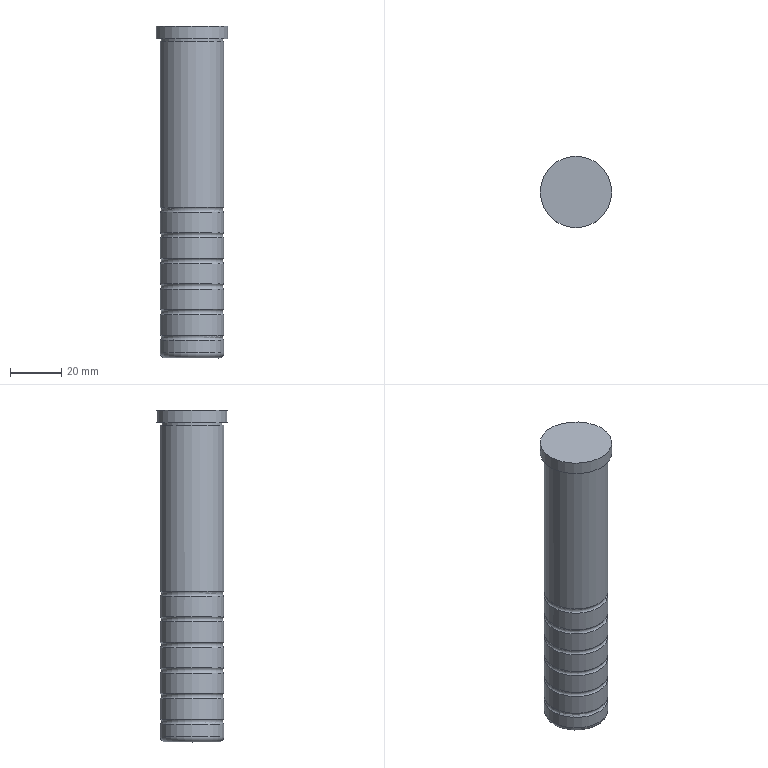Part | NX | features SGOH25-130 2 | 1 solid | 20 faces | box 28 x 28 x 130 mm | volume 64011 mm3 | cylinder 9 | torus 7 | plane 4 | commonest cylinder face diameters 25 x7 24 x1 28 x1
STEP:
#1=CARTESIAN_POINT('',(3690.594,-749.195,874.716));
#2=VERTEX_POINT('',#1);
#3=CARTESIAN_POINT('',(3703.094,-749.122,874.716));
#4=DIRECTION('',(0.,0.,1.));
#5=DIRECTION('',(1.,0.,0.));
#6=AXIS2_PLACEMENT_3D('',#3,#4,#5);
#7=CIRCLE('',#6,12.5);
#8=EDGE_CURVE('',#2,#2,#7,.T.);
#9=ORIENTED_EDGE('',*,*,#8,.T.);
#10=EDGE_LOOP('',(#9));
#11=FACE_BOUND('',#10,.T.);
#12=CARTESIAN_POINT('',(3690.594,-749.122,939.716));
#13=VERTEX_POINT('',#12);
#14=CARTESIAN_POINT('',(3703.094,-749.122,939.716));
#15=DIRECTION('',(0.,0.,-1.));
#16=DIRECTION('',(-1.,0.,0.));
#17=AXIS2_PLACEMENT_3D('',#14,#15,#16);
#18=CIRCLE('',#17,12.5);
#19=EDGE_CURVE('',#13,#13,#18,.T.);
#20=ORIENTED_EDGE('',*,*,#19,.T.);
#21=EDGE_LOOP('',(#20));
#22=FACE_BOUND('',#21,.T.);
#23=CARTESIAN_POINT('',(3703.094,-749.122,880.716));
#24=DIRECTION('',(0.,0.,-1.));
#25=DIRECTION('',(0.008727,-1.,0.));
#26=AXIS2_PLACEMENT_3D('',#23,#24,#25);
#27=CYLINDRICAL_SURFACE('',#26,12.5);
#28=ADVANCED_FACE('',(#11,#22),#27,.T.);
#29=CARTESIAN_POINT('',(3691.094,-749.122,940.716));
#30=VERTEX_POINT('',#29);
#31=CARTESIAN_POINT('',(3703.094,-749.122,940.716));
#32=DIRECTION('',(0.,0.,-1.));
#33=DIRECTION('',(-1.,0.,0.));
#34=AXIS2_PLACEMENT_3D('',#31,#32,#33);
#35=CIRCLE('',#34,12.);
#36=EDGE_CURVE('',#30,#30,#35,.T.);
#37=ORIENTED_EDGE('',*,*,#36,.T.);
#38=CARTESIAN_POINT('',(3691.094,-749.122,939.716));
#39=VERTEX_POINT('',#38);
#40=CARTESIAN_POINT('',(3691.094,-749.122,940.216));
#41=DIRECTION('',(0.,0.,-1.));
#42=VECTOR('',#41,1000.);
#43=LINE('',#40,#42);
#44=EDGE_CURVE('',#30,#39,#43,.T.);
#45=ORIENTED_EDGE('',*,*,#44,.T.);
#46=CARTESIAN_POINT('',(3703.094,-749.122,939.716));
#47=DIRECTION('',(0.,0.,1.));
#48=DIRECTION('',(-1.,0.,0.));
#49=AXIS2_PLACEMENT_3D('',#46,#47,#48);
#50=CIRCLE('',#49,12.);
#51=EDGE_CURVE('',#39,#39,#50,.T.);
#52=ORIENTED_EDGE('',*,*,#51,.T.);
#53=ORIENTED_EDGE('',*,*,#44,.F.);
#54=EDGE_LOOP('',(#37,#45,#52,#53));
#55=FACE_BOUND('',#54,.T.);
#56=CARTESIAN_POINT('',(3703.094,-749.122,940.216));
#57=DIRECTION('',(0.,0.,-1.));
#58=DIRECTION('',(1.,0.,0.));
#59=AXIS2_PLACEMENT_3D('',#56,#57,#58);
#60=CYLINDRICAL_SURFACE('',#59,12.);
#61=ADVANCED_FACE('',(#55),#60,.T.);
#62=ORIENTED_EDGE('',*,*,#19,.F.);
#63=EDGE_LOOP('',(#62));
#64=FACE_BOUND('',#63,.T.);
#65=ORIENTED_EDGE('',*,*,#51,.F.);
#66=EDGE_LOOP('',(#65));
#67=FACE_BOUND('',#66,.T.);
#68=CARTESIAN_POINT('',(3731.844,-775.103,939.716));
#69=DIRECTION('',(0.,0.,-1.));
#70=DIRECTION('',(1.,0.,0.));
#71=AXIS2_PLACEMENT_3D('',#68,#69,#70);
#72=PLANE('',#71);
#73=ADVANCED_FACE('',(#64,#67),#72,.F.);
#74=CARTESIAN_POINT('',(3690.594,-749.122,817.716));
#75=VERTEX_POINT('',#74);
#76=CARTESIAN_POINT('',(3703.094,-749.122,817.716));
#77=DIRECTION('',(0.,0.,-1.));
#78=DIRECTION('',(-1.,0.,0.));
#79=AXIS2_PLACEMENT_3D('',#76,#77,#78);
#80=CIRCLE('',#79,12.5);
#81=EDGE_CURVE('',#75,#75,#80,.T.);
#82=ORIENTED_EDGE('',*,*,#81,.T.);
#83=CARTESIAN_POINT('',(3692.594,-749.122,815.716));
#84=VERTEX_POINT('',#83);
#85=CARTESIAN_POINT('',(3692.594,-749.122,817.716));
#86=DIRECTION('',(0.,-1.,0.));
#87=DIRECTION('',(0.,0.,1.));
#88=AXIS2_PLACEMENT_3D('',#85,#86,#87);
#89=CIRCLE('',#88,2.);
#90=EDGE_CURVE('',#75,#84,#89,.T.);
#91=ORIENTED_EDGE('',*,*,#90,.T.);
#92=CARTESIAN_POINT('',(3703.094,-749.122,815.716));
#93=DIRECTION('',(0.,0.,1.));
#94=DIRECTION('',(-1.,0.,0.));
#95=AXIS2_PLACEMENT_3D('',#92,#93,#94);
#96=CIRCLE('',#95,10.5);
#97=EDGE_CURVE('',#84,#84,#96,.T.);
#98=ORIENTED_EDGE('',*,*,#97,.T.);
#99=ORIENTED_EDGE('',*,*,#90,.F.);
#100=EDGE_LOOP('',(#82,#91,#98,#99));
#101=FACE_BOUND('',#100,.T.);
#102=CARTESIAN_POINT('',(3703.094,-749.122,817.716));
#103=DIRECTION('',(0.,0.,-1.));
#104=DIRECTION('',(1.,0.,0.));
#105=AXIS2_PLACEMENT_3D('',#102,#103,#104);
#106=TOROIDAL_SURFACE('',#105,10.5,2.);
#107=ADVANCED_FACE('',(#101),#106,.T.);
#108=CARTESIAN_POINT('',(3715.594,-749.122,822.716));
#109=VERTEX_POINT('',#108);
#110=CARTESIAN_POINT('',(3690.594,-749.122,822.716));
#111=VERTEX_POINT('',#110);
#112=CARTESIAN_POINT('',(3703.094,-749.122,822.716));
#113=DIRECTION('',(0.,0.,-1.));
#114=DIRECTION('',(1.,0.,0.));
#115=AXIS2_PLACEMENT_3D('',#112,#113,#114);
#116=CIRCLE('',#115,12.5);
#117=EDGE_CURVE('',#109,#111,#116,.T.);
#118=ORIENTED_EDGE('',*,*,#117,.T.);
#119=CARTESIAN_POINT('',(3690.594,-749.122,820.216));
#120=DIRECTION('',(0.,0.,-1.));
#121=VECTOR('',#120,1000.);
#122=LINE('',#119,#121);
#123=EDGE_CURVE('',#111,#75,#122,.T.);
#124=ORIENTED_EDGE('',*,*,#123,.T.);
#125=ORIENTED_EDGE('',*,*,#81,.F.);
#126=ORIENTED_EDGE('',*,*,#123,.F.);
#127=CARTESIAN_POINT('',(3703.094,-749.122,822.716));
#128=DIRECTION('',(0.,0.,-1.));
#129=DIRECTION('',(1.,0.,0.));
#130=AXIS2_PLACEMENT_3D('',#127,#128,#129);
#131=CIRCLE('',#130,12.5);
#132=EDGE_CURVE('',#111,#109,#131,.T.);
#133=ORIENTED_EDGE('',*,*,#132,.T.);
#134=EDGE_LOOP('',(#118,#124,#125,#126,#133));
#135=FACE_BOUND('',#134,.T.);
#136=CARTESIAN_POINT('',(3703.094,-749.122,880.716));
#137=DIRECTION('',(0.,0.,-1.));
#138=DIRECTION('',(1.,0.,0.));
#139=AXIS2_PLACEMENT_3D('',#136,#137,#138);
#140=CYLINDRICAL_SURFACE('',#139,12.5);
#141=ADVANCED_FACE('',(#135),#140,.T.);
#142=ORIENTED_EDGE('',*,*,#97,.F.);
#143=EDGE_LOOP('',(#142));
#144=FACE_BOUND('',#143,.T.);
#145=CARTESIAN_POINT('',(3727.244,-770.946,815.716));
#146=DIRECTION('',(0.,0.,-1.));
#147=DIRECTION('',(1.,0.,0.));
#148=AXIS2_PLACEMENT_3D('',#145,#146,#147);
#149=PLANE('',#148);
#150=ADVANCED_FACE('',(#144),#149,.T.);
#151=CARTESIAN_POINT('',(3690.594,-749.195,872.716));
#152=VERTEX_POINT('',#151);
#153=CARTESIAN_POINT('',(3715.594,-749.122,872.716));
#154=VERTEX_POINT('',#153);
#155=CARTESIAN_POINT('',(3703.094,-749.122,872.716));
#156=DIRECTION('',(0.,0.,-1.));
#157=DIRECTION('',(1.,0.,0.));
#158=AXIS2_PLACEMENT_3D('',#155,#156,#157);
#159=CIRCLE('',#158,12.5);
#160=EDGE_CURVE('',#152,#154,#159,.T.);
#161=ORIENTED_EDGE('',*,*,#160,.F.);
#162=CARTESIAN_POINT('',(3689.844,-749.199,873.716));
#163=DIRECTION('',(0.005818,-1.,0.));
#164=DIRECTION('',(1.,0.005818,0.));
#165=AXIS2_PLACEMENT_3D('',#162,#163,#164);
#166=CIRCLE('',#165,1.25);
#167=EDGE_CURVE('',#152,#2,#166,.T.);
#168=ORIENTED_EDGE('',*,*,#167,.T.);
#169=ORIENTED_EDGE('',*,*,#8,.F.);
#170=ORIENTED_EDGE('',*,*,#167,.F.);
#171=CARTESIAN_POINT('',(3702.985,-761.622,872.716));
#172=VERTEX_POINT('',#171);
#173=CARTESIAN_POINT('',(3703.094,-749.122,872.716));
#174=DIRECTION('',(0.,0.,-1.));
#175=DIRECTION('',(1.,0.,0.));
#176=AXIS2_PLACEMENT_3D('',#173,#174,#175);
#177=CIRCLE('',#176,12.5);
#178=EDGE_CURVE('',#172,#152,#177,.T.);
#179=ORIENTED_EDGE('',*,*,#178,.F.);
#180=CARTESIAN_POINT('',(3703.094,-749.122,872.716));
#181=DIRECTION('',(0.,0.,-1.));
#182=DIRECTION('',(1.,0.,0.));
#183=AXIS2_PLACEMENT_3D('',#180,#181,#182);
#184=CIRCLE('',#183,12.5);
#185=EDGE_CURVE('',#154,#172,#184,.T.);
#186=ORIENTED_EDGE('',*,*,#185,.F.);
#187=EDGE_LOOP('',(#161,#168,#169,#170,#179,#186));
#188=FACE_BOUND('',#187,.T.);
#189=CARTESIAN_POINT('',(3703.094,-749.122,873.716));
#190=DIRECTION('',(0.,0.,1.));
#191=DIRECTION('',(-1.,0.,0.));
#192=AXIS2_PLACEMENT_3D('',#189,#190,#191);
#193=TOROIDAL_SURFACE('',#192,13.25,1.25);
#194=ADVANCED_FACE('',(#188),#193,.F.);
#195=CARTESIAN_POINT('',(3690.594,-749.122,862.716));
#196=VERTEX_POINT('',#195);
#197=CARTESIAN_POINT('',(3715.594,-749.122,862.716));
#198=VERTEX_POINT('',#197);
#199=CARTESIAN_POINT('',(3703.094,-749.122,862.716));
#200=DIRECTION('',(0.,0.,-1.));
#201=DIRECTION('',(1.,0.,0.));
#202=AXIS2_PLACEMENT_3D('',#199,#200,#201);
#203=CIRCLE('',#202,12.5);
#204=EDGE_CURVE('',#196,#198,#203,.T.);
#205=ORIENTED_EDGE('',*,*,#204,.F.);
#206=CARTESIAN_POINT('',(3690.594,-749.122,864.716));
#207=VERTEX_POINT('',#206);
#208=CARTESIAN_POINT('',(3689.844,-749.122,863.716));
#209=DIRECTION('',(0.,-1.,0.));
#210=DIRECTION('',(1.,0.,0.));
#211=AXIS2_PLACEMENT_3D('',#208,#209,#210);
#212=CIRCLE('',#211,1.25);
#213=EDGE_CURVE('',#196,#207,#212,.T.);
#214=ORIENTED_EDGE('',*,*,#213,.T.);
#215=CARTESIAN_POINT('',(3715.594,-749.122,864.716));
#216=VERTEX_POINT('',#215);
#217=CARTESIAN_POINT('',(3703.094,-749.122,864.716));
#218=DIRECTION('',(0.,0.,1.));
#219=DIRECTION('',(1.,0.,0.));
#220=AXIS2_PLACEMENT_3D('',#217,#218,#219);
#221=CIRCLE('',#220,12.5);
#222=EDGE_CURVE('',#216,#207,#221,.T.);
#223=ORIENTED_EDGE('',*,*,#222,.F.);
#224=CARTESIAN_POINT('',(3702.985,-761.622,864.716));
#225=VERTEX_POINT('',#224);
#226=CARTESIAN_POINT('',(3703.094,-749.122,864.716));
#227=DIRECTION('',(0.,0.,1.));
#228=DIRECTION('',(1.,0.,0.));
#229=AXIS2_PLACEMENT_3D('',#226,#227,#228);
#230=CIRCLE('',#229,12.5);
#231=EDGE_CURVE('',#225,#216,#230,.T.);
#232=ORIENTED_EDGE('',*,*,#231,.F.);
#233=CARTESIAN_POINT('',(3703.094,-749.122,864.716));
#234=DIRECTION('',(0.,0.,1.));
#235=DIRECTION('',(1.,0.,0.));
#236=AXIS2_PLACEMENT_3D('',#233,#234,#235);
#237=CIRCLE('',#236,12.5);
#238=EDGE_CURVE('',#207,#225,#237,.T.);
#239=ORIENTED_EDGE('',*,*,#238,.F.);
#240=ORIENTED_EDGE('',*,*,#213,.F.);
#241=CARTESIAN_POINT('',(3702.985,-761.622,862.716));
#242=VERTEX_POINT('',#241);
#243=CARTESIAN_POINT('',(3703.094,-749.122,862.716));
#244=DIRECTION('',(0.,0.,-1.));
#245=DIRECTION('',(1.,0.,0.));
#246=AXIS2_PLACEMENT_3D('',#243,#244,#245);
#247=CIRCLE('',#246,12.5);
#248=EDGE_CURVE('',#242,#196,#247,.T.);
#249=ORIENTED_EDGE('',*,*,#248,.F.);
#250=CARTESIAN_POINT('',(3703.094,-749.122,862.716));
#251=DIRECTION('',(0.,0.,-1.));
#252=DIRECTION('',(1.,0.,0.));
#253=AXIS2_PLACEMENT_3D('',#250,#251,#252);
#254=CIRCLE('',#253,12.5);
#255=EDGE_CURVE('',#198,#242,#254,.T.);
#256=ORIENTED_EDGE('',*,*,#255,.F.);
#257=EDGE_LOOP('',(#205,#214,#223,#232,#239,#240,#249,#256));
#258=FACE_BOUND('',#257,.T.);
#259=CARTESIAN_POINT('',(3703.094,-749.122,863.716));
#260=DIRECTION('',(0.,0.,1.));
#261=DIRECTION('',(0.,1.,0.));
#262=AXIS2_PLACEMENT_3D('',#259,#260,#261);
#263=TOROIDAL_SURFACE('',#262,13.25,1.25);
#264=ADVANCED_FACE('',(#258),#263,.F.);
#265=ORIENTED_EDGE('',*,*,#185,.T.);
#266=CARTESIAN_POINT('',(3702.985,-761.622,868.716));
#267=DIRECTION('',(0.,0.,-1.));
#268=VECTOR('',#267,1000.);
#269=LINE('',#266,#268);
#270=EDGE_CURVE('',#172,#225,#269,.T.);
#271=ORIENTED_EDGE('',*,*,#270,.T.);
#272=ORIENTED_EDGE('',*,*,#231,.T.);
#273=ORIENTED_EDGE('',*,*,#222,.T.);
#274=ORIENTED_EDGE('',*,*,#238,.T.);
#275=ORIENTED_EDGE('',*,*,#270,.F.);
#276=ORIENTED_EDGE('',*,*,#178,.T.);
#277=ORIENTED_EDGE('',*,*,#160,.T.);
#278=EDGE_LOOP('',(#265,#271,#272,#273,#274,#275,#276,#277));
#279=FACE_BOUND('',#278,.T.);
#280=CARTESIAN_POINT('',(3703.094,-749.122,880.716));
#281=DIRECTION('',(0.,0.,-1.));
#282=DIRECTION('',(0.008727,1.,0.));
#283=AXIS2_PLACEMENT_3D('',#280,#281,#282);
#284=CYLINDRICAL_SURFACE('',#283,12.5);
#285=ADVANCED_FACE('',(#279),#284,.T.);
#286=CARTESIAN_POINT('',(3690.594,-749.122,852.716));
#287=VERTEX_POINT('',#286);
#288=CARTESIAN_POINT('',(3715.594,-749.122,852.716));
#289=VERTEX_POINT('',#288);
#290=CARTESIAN_POINT('',(3703.094,-749.122,852.716));
#291=DIRECTION('',(0.,0.,-1.));
#292=DIRECTION('',(1.,0.,0.));
#293=AXIS2_PLACEMENT_3D('',#290,#291,#292);
#294=CIRCLE('',#293,12.5);
#295=EDGE_CURVE('',#287,#289,#294,.T.);
#296=ORIENTED_EDGE('',*,*,#295,.F.);
#297=CARTESIAN_POINT('',(3690.594,-749.122,854.716));
#298=VERTEX_POINT('',#297);
#299=CARTESIAN_POINT('',(3689.844,-749.122,853.716));
#300=DIRECTION('',(0.,-1.,0.));
#301=DIRECTION('',(1.,0.,0.));
#302=AXIS2_PLACEMENT_3D('',#299,#300,#301);
#303=CIRCLE('',#302,1.25);
#304=EDGE_CURVE('',#287,#298,#303,.T.);
#305=ORIENTED_EDGE('',*,*,#304,.T.);
#306=CARTESIAN_POINT('',(3715.594,-749.122,854.716));
#307=VERTEX_POINT('',#306);
#308=CARTESIAN_POINT('',(3703.094,-749.122,854.716));
#309=DIRECTION('',(0.,0.,1.));
#310=DIRECTION('',(1.,0.,0.));
#311=AXIS2_PLACEMENT_3D('',#308,#309,#310);
#312=CIRCLE('',#311,12.5);
#313=EDGE_CURVE('',#307,#298,#312,.T.);
#314=ORIENTED_EDGE('',*,*,#313,.F.);
#315=CARTESIAN_POINT('',(3702.985,-761.622,854.716));
#316=VERTEX_POINT('',#315);
#317=CARTESIAN_POINT('',(3703.094,-749.122,854.716));
#318=DIRECTION('',(0.,0.,1.));
#319=DIRECTION('',(1.,0.,0.));
#320=AXIS2_PLACEMENT_3D('',#317,#318,#319);
#321=CIRCLE('',#320,12.5);
#322=EDGE_CURVE('',#316,#307,#321,.T.);
#323=ORIENTED_EDGE('',*,*,#322,.F.);
#324=CARTESIAN_POINT('',(3703.094,-749.122,854.716));
#325=DIRECTION('',(0.,0.,1.));
#326=DIRECTION('',(1.,0.,0.));
#327=AXIS2_PLACEMENT_3D('',#324,#325,#326);
#328=CIRCLE('',#327,12.5);
#329=EDGE_CURVE('',#298,#316,#328,.T.);
#330=ORIENTED_EDGE('',*,*,#329,.F.);
#331=ORIENTED_EDGE('',*,*,#304,.F.);
#332=CARTESIAN_POINT('',(3702.985,-761.622,852.716));
#333=VERTEX_POINT('',#332);
#334=CARTESIAN_POINT('',(3703.094,-749.122,852.716));
#335=DIRECTION('',(0.,0.,-1.));
#336=DIRECTION('',(1.,0.,0.));
#337=AXIS2_PLACEMENT_3D('',#334,#335,#336);
#338=CIRCLE('',#337,12.5);
#339=EDGE_CURVE('',#333,#287,#338,.T.);
#340=ORIENTED_EDGE('',*,*,#339,.F.);
#341=CARTESIAN_POINT('',(3703.094,-749.122,852.716));
#342=DIRECTION('',(0.,0.,-1.));
#343=DIRECTION('',(1.,0.,0.));
#344=AXIS2_PLACEMENT_3D('',#341,#342,#343);
#345=CIRCLE('',#344,12.5);
#346=EDGE_CURVE('',#289,#333,#345,.T.);
#347=ORIENTED_EDGE('',*,*,#346,.F.);
#348=EDGE_LOOP('',(#296,#305,#314,#323,#330,#331,#340,#347));
#349=FACE_BOUND('',#348,.T.);
#350=CARTESIAN_POINT('',(3703.094,-749.122,853.716));
#351=DIRECTION('',(0.,0.,1.));
#352=DIRECTION('',(-1.,0.,0.));
#353=AXIS2_PLACEMENT_3D('',#350,#351,#352);
#354=TOROIDAL_SURFACE('',#353,13.25,1.25);
#355=ADVANCED_FACE('',(#349),#354,.F.);
#356=ORIENTED_EDGE('',*,*,#255,.T.);
#357=CARTESIAN_POINT('',(3702.985,-761.622,858.716));
#358=DIRECTION('',(0.,0.,-1.));
#359=VECTOR('',#358,1000.);
#360=LINE('',#357,#359);
#361=EDGE_CURVE('',#242,#316,#360,.T.);
#362=ORIENTED_EDGE('',*,*,#361,.T.);
#363=ORIENTED_EDGE('',*,*,#322,.T.);
#364=ORIENTED_EDGE('',*,*,#313,.T.);
#365=ORIENTED_EDGE('',*,*,#329,.T.);
#366=ORIENTED_EDGE('',*,*,#361,.F.);
#367=ORIENTED_EDGE('',*,*,#248,.T.);
#368=ORIENTED_EDGE('',*,*,#204,.T.);
#369=EDGE_LOOP('',(#356,#362,#363,#364,#365,#366,#367,#368));
#370=FACE_BOUND('',#369,.T.);
#371=CARTESIAN_POINT('',(3703.094,-749.122,880.716));
#372=DIRECTION('',(0.,0.,-1.));
#373=DIRECTION('',(0.008727,1.,0.));
#374=AXIS2_PLACEMENT_3D('',#371,#372,#373);
#375=CYLINDRICAL_SURFACE('',#374,12.5);
#376=ADVANCED_FACE('',(#370),#375,.T.);
#377=CARTESIAN_POINT('',(3690.594,-749.122,842.716));
#378=VERTEX_POINT('',#377);
#379=CARTESIAN_POINT('',(3715.594,-749.122,842.716));
#380=VERTEX_POINT('',#379);
#381=CARTESIAN_POINT('',(3703.094,-749.122,842.716));
#382=DIRECTION('',(0.,0.,-1.));
#383=DIRECTION('',(1.,0.,0.));
#384=AXIS2_PLACEMENT_3D('',#381,#382,#383);
#385=CIRCLE('',#384,12.5);
#386=EDGE_CURVE('',#378,#380,#385,.T.);
#387=ORIENTED_EDGE('',*,*,#386,.F.);
#388=CARTESIAN_POINT('',(3690.594,-749.122,844.716));
#389=VERTEX_POINT('',#388);
#390=CARTESIAN_POINT('',(3689.844,-749.122,843.716));
#391=DIRECTION('',(0.,-1.,0.));
#392=DIRECTION('',(1.,0.,0.));
#393=AXIS2_PLACEMENT_3D('',#390,#391,#392);
#394=CIRCLE('',#393,1.25);
#395=EDGE_CURVE('',#378,#389,#394,.T.);
#396=ORIENTED_EDGE('',*,*,#395,.T.);
#397=CARTESIAN_POINT('',(3715.594,-749.122,844.716));
#398=VERTEX_POINT('',#397);
#399=CARTESIAN_POINT('',(3703.094,-749.122,844.716));
#400=DIRECTION('',(0.,0.,1.));
#401=DIRECTION('',(1.,0.,0.));
#402=AXIS2_PLACEMENT_3D('',#399,#400,#401);
#403=CIRCLE('',#402,12.5);
#404=EDGE_CURVE('',#398,#389,#403,.T.);
#405=ORIENTED_EDGE('',*,*,#404,.F.);
#406=CARTESIAN_POINT('',(3702.985,-761.622,844.716));
#407=VERTEX_POINT('',#406);
#408=CARTESIAN_POINT('',(3703.094,-749.122,844.716));
#409=DIRECTION('',(0.,0.,1.));
#410=DIRECTION('',(1.,0.,0.));
#411=AXIS2_PLACEMENT_3D('',#408,#409,#410);
#412=CIRCLE('',#411,12.5);
#413=EDGE_CURVE('',#407,#398,#412,.T.);
#414=ORIENTED_EDGE('',*,*,#413,.F.);
#415=CARTESIAN_POINT('',(3703.094,-749.122,844.716));
#416=DIRECTION('',(0.,0.,1.));
#417=DIRECTION('',(1.,0.,0.));
#418=AXIS2_PLACEMENT_3D('',#415,#416,#417);
#419=CIRCLE('',#418,12.5);
#420=EDGE_CURVE('',#389,#407,#419,.T.);
#421=ORIENTED_EDGE('',*,*,#420,.F.);
#422=ORIENTED_EDGE('',*,*,#395,.F.);
#423=CARTESIAN_POINT('',(3702.985,-761.622,842.716));
#424=VERTEX_POINT('',#423);
#425=CARTESIAN_POINT('',(3703.094,-749.122,842.716));
#426=DIRECTION('',(0.,0.,-1.));
#427=DIRECTION('',(1.,0.,0.));
#428=AXIS2_PLACEMENT_3D('',#425,#426,#427);
#429=CIRCLE('',#428,12.5);
#430=EDGE_CURVE('',#424,#378,#429,.T.);
#431=ORIENTED_EDGE('',*,*,#430,.F.);
#432=CARTESIAN_POINT('',(3703.094,-749.122,842.716));
#433=DIRECTION('',(0.,0.,-1.));
#434=DIRECTION('',(1.,0.,0.));
#435=AXIS2_PLACEMENT_3D('',#432,#433,#434);
#436=CIRCLE('',#435,12.5);
#437=EDGE_CURVE('',#380,#424,#436,.T.);
#438=ORIENTED_EDGE('',*,*,#437,.F.);
#439=EDGE_LOOP('',(#387,#396,#405,#414,#421,#422,#431,#438));
#440=FACE_BOUND('',#439,.T.);
#441=CARTESIAN_POINT('',(3703.094,-749.122,843.716));
#442=DIRECTION('',(0.,0.,1.));
#443=DIRECTION('',(-1.,0.,0.));
#444=AXIS2_PLACEMENT_3D('',#441,#442,#443);
#445=TOROIDAL_SURFACE('',#444,13.25,1.25);
#446=ADVANCED_FACE('',(#440),#445,.F.);
#447=ORIENTED_EDGE('',*,*,#346,.T.);
#448=CARTESIAN_POINT('',(3702.985,-761.622,848.716));
#449=DIRECTION('',(0.,0.,-1.));
#450=VECTOR('',#449,1000.);
#451=LINE('',#448,#450);
#452=EDGE_CURVE('',#333,#407,#451,.T.);
#453=ORIENTED_EDGE('',*,*,#452,.T.);
#454=ORIENTED_EDGE('',*,*,#413,.T.);
#455=ORIENTED_EDGE('',*,*,#404,.T.);
#456=ORIENTED_EDGE('',*,*,#420,.T.);
#457=ORIENTED_EDGE('',*,*,#452,.F.);
#458=ORIENTED_EDGE('',*,*,#339,.T.);
#459=ORIENTED_EDGE('',*,*,#295,.T.);
#460=EDGE_LOOP('',(#447,#453,#454,#455,#456,#457,#458,#459));
#461=FACE_BOUND('',#460,.T.);
#462=CARTESIAN_POINT('',(3703.094,-749.122,880.716));
#463=DIRECTION('',(0.,0.,-1.));
#464=DIRECTION('',(0.008727,1.,0.));
#465=AXIS2_PLACEMENT_3D('',#462,#463,#464);
#466=CYLINDRICAL_SURFACE('',#465,12.5);
#467=ADVANCED_FACE('',(#461),#466,.T.);
#468=CARTESIAN_POINT('',(3690.594,-749.122,832.716));
#469=VERTEX_POINT('',#468);
#470=CARTESIAN_POINT('',(3715.594,-749.122,832.716));
#471=VERTEX_POINT('',#470);
#472=CARTESIAN_POINT('',(3703.094,-749.122,832.716));
#473=DIRECTION('',(0.,0.,-1.));
#474=DIRECTION('',(1.,0.,0.));
#475=AXIS2_PLACEMENT_3D('',#472,#473,#474);
#476=CIRCLE('',#475,12.5);
#477=EDGE_CURVE('',#469,#471,#476,.T.);
#478=ORIENTED_EDGE('',*,*,#477,.F.);
#479=CARTESIAN_POINT('',(3690.594,-749.122,834.716));
#480=VERTEX_POINT('',#479);
#481=CARTESIAN_POINT('',(3689.844,-749.122,833.716));
#482=DIRECTION('',(0.,-1.,0.));
#483=DIRECTION('',(1.,0.,0.));
#484=AXIS2_PLACEMENT_3D('',#481,#482,#483);
#485=CIRCLE('',#484,1.25);
#486=EDGE_CURVE('',#469,#480,#485,.T.);
#487=ORIENTED_EDGE('',*,*,#486,.T.);
#488=CARTESIAN_POINT('',(3715.594,-749.122,834.716));
#489=VERTEX_POINT('',#488);
#490=CARTESIAN_POINT('',(3703.094,-749.122,834.716));
#491=DIRECTION('',(0.,0.,1.));
#492=DIRECTION('',(1.,0.,0.));
#493=AXIS2_PLACEMENT_3D('',#490,#491,#492);
#494=CIRCLE('',#493,12.5);
#495=EDGE_CURVE('',#489,#480,#494,.T.);
#496=ORIENTED_EDGE('',*,*,#495,.F.);
#497=CARTESIAN_POINT('',(3702.985,-761.622,834.716));
#498=VERTEX_POINT('',#497);
#499=CARTESIAN_POINT('',(3703.094,-749.122,834.716));
#500=DIRECTION('',(0.,0.,1.));
#501=DIRECTION('',(1.,0.,0.));
#502=AXIS2_PLACEMENT_3D('',#499,#500,#501);
#503=CIRCLE('',#502,12.5);
#504=EDGE_CURVE('',#498,#489,#503,.T.);
#505=ORIENTED_EDGE('',*,*,#504,.F.);
#506=CARTESIAN_POINT('',(3703.094,-749.122,834.716));
#507=DIRECTION('',(0.,0.,1.));
#508=DIRECTION('',(1.,0.,0.));
#509=AXIS2_PLACEMENT_3D('',#506,#507,#508);
#510=CIRCLE('',#509,12.5);
#511=EDGE_CURVE('',#480,#498,#510,.T.);
#512=ORIENTED_EDGE('',*,*,#511,.F.);
#513=ORIENTED_EDGE('',*,*,#486,.F.);
#514=CARTESIAN_POINT('',(3702.985,-761.622,832.716));
#515=VERTEX_POINT('',#514);
#516=CARTESIAN_POINT('',(3703.094,-749.122,832.716));
#517=DIRECTION('',(0.,0.,-1.));
#518=DIRECTION('',(1.,0.,0.));
#519=AXIS2_PLACEMENT_3D('',#516,#517,#518);
#520=CIRCLE('',#519,12.5);
#521=EDGE_CURVE('',#515,#469,#520,.T.);
#522=ORIENTED_EDGE('',*,*,#521,.F.);
#523=CARTESIAN_POINT('',(3703.094,-749.122,832.716));
#524=DIRECTION('',(0.,0.,-1.));
#525=DIRECTION('',(1.,0.,0.));
#526=AXIS2_PLACEMENT_3D('',#523,#524,#525);
#527=CIRCLE('',#526,12.5);
#528=EDGE_CURVE('',#471,#515,#527,.T.);
#529=ORIENTED_EDGE('',*,*,#528,.F.);
#530=EDGE_LOOP('',(#478,#487,#496,#505,#512,#513,#522,#529));
#531=FACE_BOUND('',#530,.T.);
#532=CARTESIAN_POINT('',(3703.094,-749.122,833.716));
#533=DIRECTION('',(0.,0.,1.));
#534=DIRECTION('',(-1.,0.,0.));
#535=AXIS2_PLACEMENT_3D('',#532,#533,#534);
#536=TOROIDAL_SURFACE('',#535,13.25,1.25);
#537=ADVANCED_FACE('',(#531),#536,.F.);
#538=ORIENTED_EDGE('',*,*,#437,.T.);
#539=CARTESIAN_POINT('',(3702.985,-761.622,838.716));
#540=DIRECTION('',(0.,0.,-1.));
#541=VECTOR('',#540,1000.);
#542=LINE('',#539,#541);
#543=EDGE_CURVE('',#424,#498,#542,.T.);
#544=ORIENTED_EDGE('',*,*,#543,.T.);
#545=ORIENTED_EDGE('',*,*,#504,.T.);
#546=ORIENTED_EDGE('',*,*,#495,.T.);
#547=ORIENTED_EDGE('',*,*,#511,.T.);
#548=ORIENTED_EDGE('',*,*,#543,.F.);
#549=ORIENTED_EDGE('',*,*,#430,.T.);
#550=ORIENTED_EDGE('',*,*,#386,.T.);
#551=EDGE_LOOP('',(#538,#544,#545,#546,#547,#548,#549,#550));
#552=FACE_BOUND('',#551,.T.);
#553=CARTESIAN_POINT('',(3703.094,-749.122,880.716));
#554=DIRECTION('',(0.,0.,-1.));
#555=DIRECTION('',(0.008727,1.,0.));
#556=AXIS2_PLACEMENT_3D('',#553,#554,#555);
#557=CYLINDRICAL_SURFACE('',#556,12.5);
#558=ADVANCED_FACE('',(#552),#557,.T.);
#559=ORIENTED_EDGE('',*,*,#132,.F.);
#560=CARTESIAN_POINT('',(3690.594,-749.122,824.716));
#561=VERTEX_POINT('',#560);
#562=CARTESIAN_POINT('',(3689.844,-749.122,823.716));
#563=DIRECTION('',(0.,-1.,0.));
#564=DIRECTION('',(1.,0.,0.));
#565=AXIS2_PLACEMENT_3D('',#562,#563,#564);
#566=CIRCLE('',#565,1.25);
#567=EDGE_CURVE('',#111,#561,#566,.T.);
#568=ORIENTED_EDGE('',*,*,#567,.T.);
#569=CARTESIAN_POINT('',(3715.594,-749.122,824.716));
#570=VERTEX_POINT('',#569);
#571=CARTESIAN_POINT('',(3703.094,-749.122,824.716));
#572=DIRECTION('',(0.,0.,1.));
#573=DIRECTION('',(1.,0.,0.));
#574=AXIS2_PLACEMENT_3D('',#571,#572,#573);
#575=CIRCLE('',#574,12.5);
#576=EDGE_CURVE('',#570,#561,#575,.T.);
#577=ORIENTED_EDGE('',*,*,#576,.F.);
#578=CARTESIAN_POINT('',(3702.985,-761.622,824.716));
#579=VERTEX_POINT('',#578);
#580=CARTESIAN_POINT('',(3703.094,-749.122,824.716));
#581=DIRECTION('',(0.,0.,1.));
#582=DIRECTION('',(1.,0.,0.));
#583=AXIS2_PLACEMENT_3D('',#580,#581,#582);
#584=CIRCLE('',#583,12.5);
#585=EDGE_CURVE('',#579,#570,#584,.T.);
#586=ORIENTED_EDGE('',*,*,#585,.F.);
#587=CARTESIAN_POINT('',(3703.094,-749.122,824.716));
#588=DIRECTION('',(0.,0.,1.));
#589=DIRECTION('',(1.,0.,0.));
#590=AXIS2_PLACEMENT_3D('',#587,#588,#589);
#591=CIRCLE('',#590,12.5);
#592=EDGE_CURVE('',#561,#579,#591,.T.);
#593=ORIENTED_EDGE('',*,*,#592,.F.);
#594=ORIENTED_EDGE('',*,*,#567,.F.);
#595=ORIENTED_EDGE('',*,*,#117,.F.);
#596=EDGE_LOOP('',(#559,#568,#577,#586,#593,#594,#595));
#597=FACE_BOUND('',#596,.T.);
#598=CARTESIAN_POINT('',(3703.094,-749.122,823.716));
#599=DIRECTION('',(0.,0.,1.));
#600=DIRECTION('',(0.,1.,0.));
#601=AXIS2_PLACEMENT_3D('',#598,#599,#600);
#602=TOROIDAL_SURFACE('',#601,13.25,1.25);
#603=ADVANCED_FACE('',(#597),#602,.F.);
#604=ORIENTED_EDGE('',*,*,#528,.T.);
#605=CARTESIAN_POINT('',(3702.985,-761.622,828.716));
#606=DIRECTION('',(0.,0.,-1.));
#607=VECTOR('',#606,1000.);
#608=LINE('',#605,#607);
#609=EDGE_CURVE('',#515,#579,#608,.T.);
#610=ORIENTED_EDGE('',*,*,#609,.T.);
#611=ORIENTED_EDGE('',*,*,#585,.T.);
#612=ORIENTED_EDGE('',*,*,#576,.T.);
#613=ORIENTED_EDGE('',*,*,#592,.T.);
#614=ORIENTED_EDGE('',*,*,#609,.F.);
#615=ORIENTED_EDGE('',*,*,#521,.T.);
#616=ORIENTED_EDGE('',*,*,#477,.T.);
#617=EDGE_LOOP('',(#604,#610,#611,#612,#613,#614,#615,#616));
#618=FACE_BOUND('',#617,.T.);
#619=CARTESIAN_POINT('',(3703.094,-749.122,880.716));
#620=DIRECTION('',(0.,0.,-1.));
#621=DIRECTION('',(0.008727,1.,0.));
#622=AXIS2_PLACEMENT_3D('',#619,#620,#621);
#623=CYLINDRICAL_SURFACE('',#622,12.5);
#624=ADVANCED_FACE('',(#618),#623,.T.);
#625=CARTESIAN_POINT('',(3689.094,-749.122,940.716));
#626=VERTEX_POINT('',#625);
#627=CARTESIAN_POINT('',(3703.094,-749.122,940.716));
#628=DIRECTION('',(0.,0.,-1.));
#629=DIRECTION('',(-1.,0.,0.));
#630=AXIS2_PLACEMENT_3D('',#627,#628,#629);
#631=CIRCLE('',#630,14.);
#632=EDGE_CURVE('',#626,#626,#631,.T.);
#633=ORIENTED_EDGE('',*,*,#632,.T.);
#634=EDGE_LOOP('',(#633));
#635=FACE_BOUND('',#634,.T.);
#636=ORIENTED_EDGE('',*,*,#36,.F.);
#637=EDGE_LOOP('',(#636));
#638=FACE_BOUND('',#637,.T.);
#639=CARTESIAN_POINT('',(3735.294,-778.22,940.716));
#640=DIRECTION('',(0.,0.,-1.));
#641=DIRECTION('',(1.,0.,0.));
#642=AXIS2_PLACEMENT_3D('',#639,#640,#641);
#643=PLANE('',#642);
#644=ADVANCED_FACE('',(#635,#638),#643,.T.);
#645=CARTESIAN_POINT('',(3689.094,-749.122,945.716));
#646=VERTEX_POINT('',#645);
#647=CARTESIAN_POINT('',(3703.094,-749.122,945.716));
#648=DIRECTION('',(0.,0.,1.));
#649=DIRECTION('',(-1.,0.,0.));
#650=AXIS2_PLACEMENT_3D('',#647,#648,#649);
#651=CIRCLE('',#650,14.);
#652=EDGE_CURVE('',#646,#646,#651,.T.);
#653=ORIENTED_EDGE('',*,*,#652,.F.);
#654=CARTESIAN_POINT('',(3689.094,-749.122,943.216));
#655=DIRECTION('',(0.,0.,-1.));
#656=VECTOR('',#655,1000.);
#657=LINE('',#654,#656);
#658=EDGE_CURVE('',#646,#626,#657,.T.);
#659=ORIENTED_EDGE('',*,*,#658,.T.);
#660=ORIENTED_EDGE('',*,*,#632,.F.);
#661=ORIENTED_EDGE('',*,*,#658,.F.);
#662=EDGE_LOOP('',(#653,#659,#660,#661));
#663=FACE_BOUND('',#662,.T.);
#664=CARTESIAN_POINT('',(3703.094,-749.122,943.216));
#665=DIRECTION('',(0.,0.,-1.));
#666=DIRECTION('',(1.,0.,0.));
#667=AXIS2_PLACEMENT_3D('',#664,#665,#666);
#668=CYLINDRICAL_SURFACE('',#667,14.);
#669=ADVANCED_FACE('',(#663),#668,.T.);
#670=ORIENTED_EDGE('',*,*,#652,.T.);
#671=EDGE_LOOP('',(#670));
#672=FACE_BOUND('',#671,.T.);
#673=CARTESIAN_POINT('',(3684.894,-778.22,945.716));
#674=DIRECTION('',(0.,0.,1.));
#675=DIRECTION('',(-1.,0.,0.));
#676=AXIS2_PLACEMENT_3D('',#673,#674,#675);
#677=PLANE('',#676);
#678=ADVANCED_FACE('',(#672),#677,.T.);
#679=CLOSED_SHELL('',(#28,#61,#73,#107,#141,#150,#194,#264,#285,#355,#376,#446,#467,#537,#558,#603,#624,#644,#669,#678));
#680=MANIFOLD_SOLID_BREP('',#679);
#681=(LENGTH_UNIT()NAMED_UNIT(*)SI_UNIT(.MILLI.,.METRE.));
#682=UNCERTAINTY_MEASURE_WITH_UNIT(LENGTH_MEASURE(0.00001),#681,'','');
#683=(NAMED_UNIT(*)PLANE_ANGLE_UNIT()SI_UNIT($,.RADIAN.));
#684=(NAMED_UNIT(*)SI_UNIT($,.STERADIAN.)SOLID_ANGLE_UNIT());
#685=(GEOMETRIC_REPRESENTATION_CONTEXT(3)GLOBAL_UNCERTAINTY_ASSIGNED_CONTEXT((#682))GLOBAL_UNIT_ASSIGNED_CONTEXT((#681,#683,#684))REPRESENTATION_CONTEXT('',''));
#686=ADVANCED_BREP_SHAPE_REPRESENTATION('',(#680),#685);